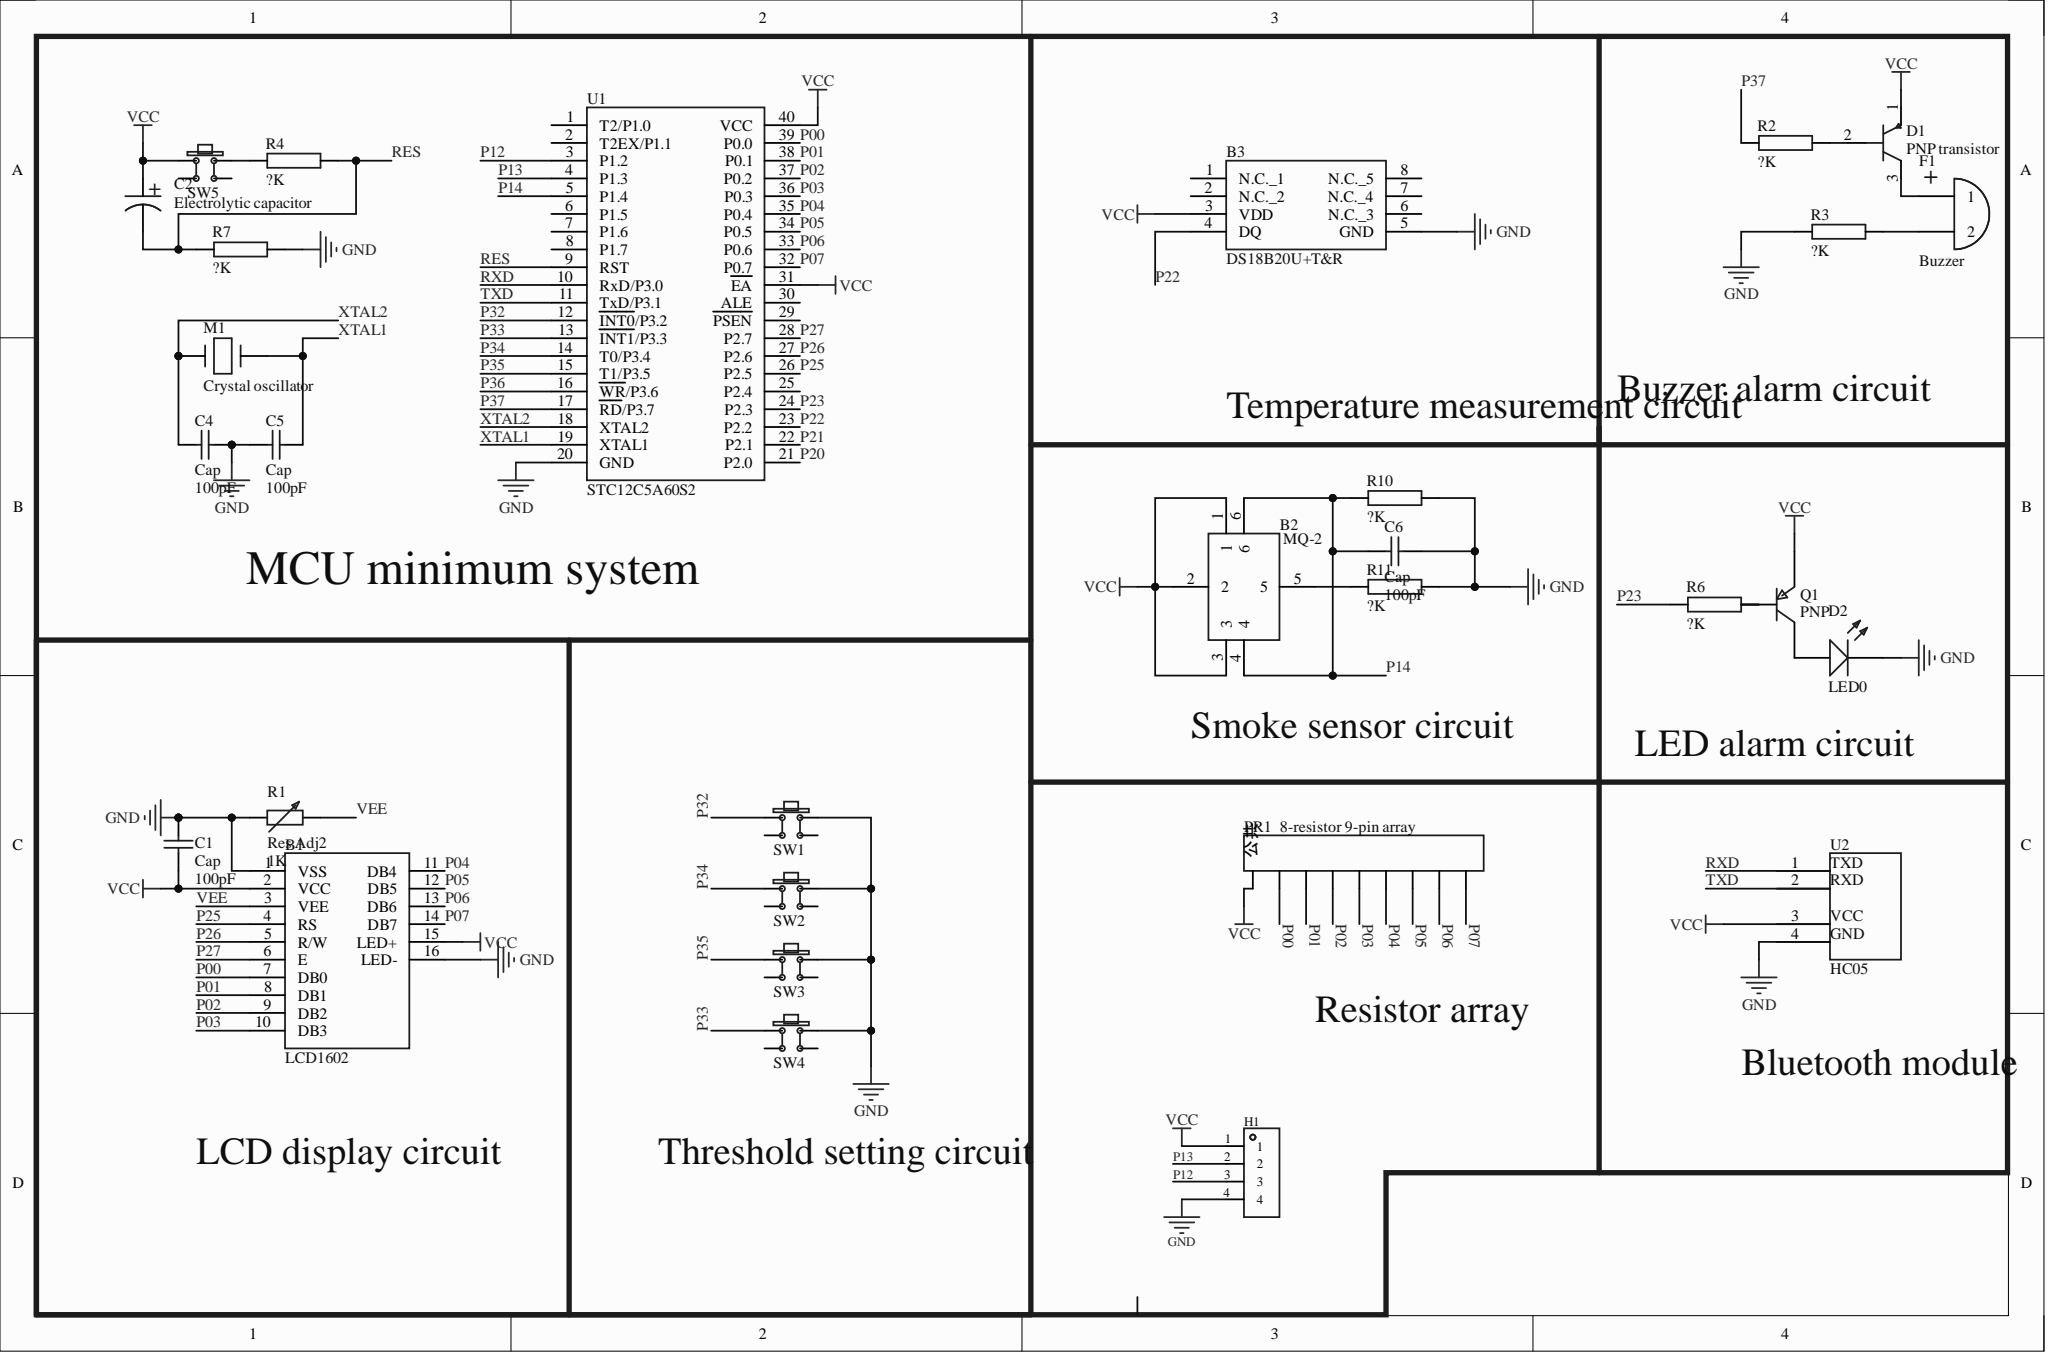Circuit board | Altium Designer | 30 parts | 36 nets
Bill of materials:
Comment,Description,Designator,Footprint,LibRef,Quantity
"LCD1602","Character LCD Module 1602 Built in Controller St7066u COB Type LCD","B1","LCD1602","LCD1602","1"
"MQ-2","Sensor: gas; smoke,combustible gases; Range: 30010000ppm; MQ-2","B2","SENSOR-TH_MQ-2","MQ-2","1"
"DS18B20U+T&R","Board Mount Temperature Sensors Prgmble Resolution 1-Wire Parasite Pwr","B3","HDR-TH_8P-P2.54-V-F-R2-C4-S2.54-1","DS18B20U+T&R","1"
"Cap","Capacitor","C1, C4, C5, C6","RAD-0.3","Cap","4"
"Electrolytic capacitor","","C2","CAP-TH_BD5.0-P2.00-D0.8-FD-10UF50VC110GL","电解电容","1"
"PNP transistor","","D1","S8550P_TO-92","PNP三极管","1"
"LED0","Typical INFRARED GaAs LED","D2","LED-TH_5mm","LED0","1"
"Buzzer","","F1","BUZ-TH_BD12.0-P6.00-D0.9-RD","蜂鸣器","1"
"","","H1","HDR-TH_4P-P2.54-V-F","HDR-F_2.54_1x4P","1"
"Crystal oscillator","","M1","HC-49S_L11.5-W5.0-P4.88","晶振","1"
"8-resistor 9-pin array","","PR1","RES-ARRAY-TH_9P-P2.54-D1.0","8阻9排","1"
"PNP","PNP Bipolar Transistor","Q1","TO-92-3_L4.6-W3.6-P1.27-L_1","PNP","1"
"Res Adj2","Variable Resistor","R1","RES-ADJ-TH_3P-L9.5-W4.85-P2.54_PV36W103C01B00","Res Adj2","1"
"?K","","R2, R3, R4, R6, R7, R10, R11","Res_1/4W","？K","7"
"TSW tactile switch","TSW tactile switch","SW1, SW2, SW3, SW4, SW5","SW-TH_4P-L6.0-W6.0-P4.50-LS6.5","TSW 轻触开关","5"
"STC12C5A60S2","STC MCU","U1","DIP-40_L52.3-W13.9-P2.54-LS15.2-BL-BASE","STC12C5A60S2","1"
"HC05","","U2","HDR-TH_4P-P2.54-V-F","HC05","1"
Netlist (Protel format):
[
B1
LCD1602
LCD1602



]
[
B2
SENSOR-TH_MQ-2
MQ-2



]
[
B3
HDR-TH_8P-P2.54-V-F-R2-C4-S2.54-1
DS18B20U+T&R



]
[
C1
RAD-0.3
Cap



]
[
C2
CAP-TH_BD5.0-P2.00-D0.8-FD-10UF50VC110GL
Electrolytic capacitor



]
[
C4
RAD-0.3
Cap



]
[
C5
RAD-0.3
Cap



]
[
C6
RAD-0.3
Cap



]
[
D1
S8550P_TO-92
PNP transistor



]
[
D2
LED-TH_5mm
LED0



]
[
F1
BUZ-TH_BD12.0-P6.00-D0.9-RD
Buzzer



]
[
H1
HDR-TH_4P-P2.54-V-F




]
[
M1
HC-49S_L11.5-W5.0-P4.88
Crystal oscillator



]
[
PR1
RES-ARRAY-TH_9P-P2.54-D1.0
8-resistor 9-pin array



]
[
Q1
TO-92-3_L4.6-W3.6-P1.27-L_1
PNP



]
[
R1
RES-ADJ-TH_3P-L9.5-W4.85-P2.54_PV36W103C01B00
Res Adj2



]
[
R2
Res_1/4W
?K



]
[
R3
Res_1/4W
?K



]
[
R4
Res_1/4W
?K



]
[
R6
Res_1/4W
?K



]
[
R7
Res_1/4W
?K



]
[
R10
Res_1/4W
?K



]
[
R11
Res_1/4W
?K



]
[
SW1
SW-TH_4P-L6.0-W6.0-P4.50-LS6.5
TSW tactile switch



]
[
SW2
SW-TH_4P-L6.0-W6.0-P4.50-LS6.5
TSW tactile switch



]
[
SW3
SW-TH_4P-L6.0-W6.0-P4.50-LS6.5
TSW tactile switch



]
[
SW4
SW-TH_4P-L6.0-W6.0-P4.50-LS6.5
TSW tactile switch



]
[
SW5
SW-TH_4P-L6.0-W6.0-P4.50-LS6.5
TSW tactile switch



]
[
U1
DIP-40_L52.3-W13.9-P2.54-LS15.2-BL-BASE
STC12C5A60S2



]
[
U2
HDR-TH_4P-P2.54-V-F
HC05



]
(
XTAL2
C4-1
M1-1
U1-18
)
(
XTAL1
C5-2
M1-2
U1-19
)
(
VEE
B1-3
R1-2
)
(
VCC
B1-2
B1-15
B2-1
B2-2
B2-3
B3-3
C1-1
C2-1
D1-1
H1-1
PR1-1
Q1-3
SW5-1
U1-31
U1-40
U2-3
)
(
TXD
U1-11
U2-2
)
(
RXD
U1-10
U2-1
)
(
RES
C2-2
R4-2
R7-1
U1-9
)
(
P37
R2-1
U1-17
)
(
P35
SW3-1
U1-15
)
(
P34
SW2-1
U1-14
)
(
P33
SW4-1
U1-13
)
(
P32
SW1-1
U1-12
)
(
P27
B1-6
U1-28
)
(
P26
B1-5
U1-27
)
(
P25
B1-4
U1-26
)
(
P23
R6-1
U1-24
)
(
P22
B3-4
U1-23
)
(
P14
B2-4
B2-6
C6-2
R10-1
U1-5
)
(
P13
H1-2
U1-4
)
(
P12
H1-3
U1-3
)
(
P07
B1-14
PR1-9
U1-32
)
(
P06
B1-13
PR1-8
U1-33
)
(
P05
B1-12
PR1-7
U1-34
)
(
P04
B1-11
PR1-6
U1-35
)
(
P03
B1-10
PR1-5
U1-36
)
(
P02
B1-9
PR1-4
U1-37
)
(
P01
B1-8
PR1-3
U1-38
)
(
P00
B1-7
PR1-2
U1-39
)
(
NetR4_1
R4-1
SW5-4
)
(
NetQ1_2
Q1-2
R6-2
)
(
NetF1_2
F1-2
R3-1
)
(
NetD2_1
D2-1
Q1-1
)
(
NetD1_3
D1-3
F1-1
)
(
NetD1_2
D1-2
R2-2
)
(
NetB2_5
B2-5
R11-1
)
(
GND
B1-1
B1-16
B3-5
C1-2
C4-2
C5-1
C6-1
D2-2
H1-4
R1-1
R3-2
R7-2
R10-2
R11-2
SW1-4
SW2-4
SW3-4
SW4-4
U1-20
U2-4
)